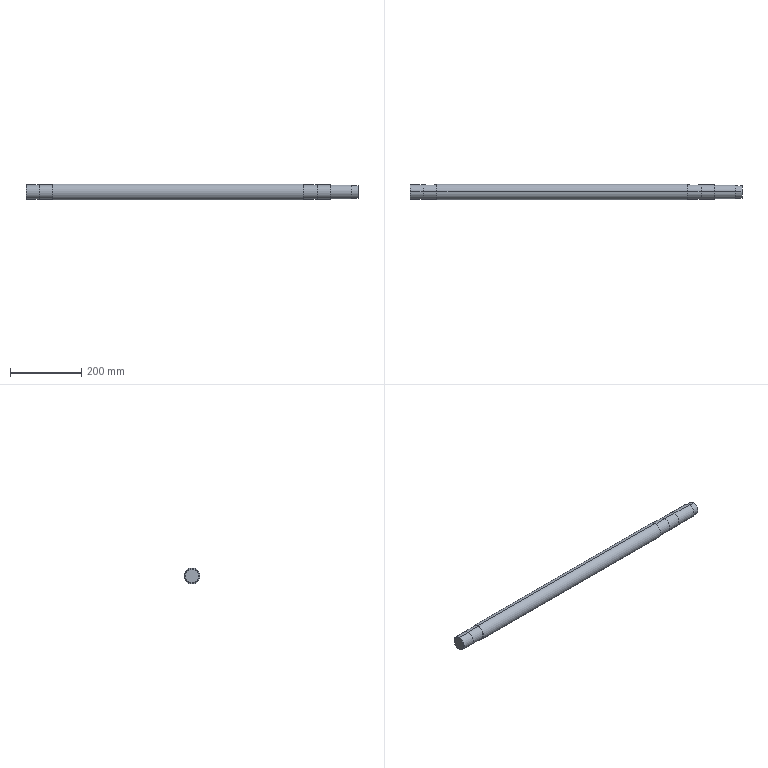Part | SolidWorks | features ICE 8, Chamfer 1, Extrusion 1, HoleWzd 1 | 1 solid | 43 faces | box 935 x 45 x 45 mm | volume 1400628 mm3 | cylinder 22 | plane 17 | cone 4 | commonest cylinder face diameters 12 x4 40 x4 41 x4 8.5 x2 10 x2 35 x2
STEP:
#1=CARTESIAN_POINT('',(844.,0.,4.25));
#2=VERTEX_POINT('',#1);
#3=CARTESIAN_POINT('',(844.,0.,-4.25));
#4=VERTEX_POINT('',#3);
#5=CARTESIAN_POINT('',(844.,0.,0.));
#6=DIRECTION('',(1.,0.,0.));
#7=DIRECTION('',(0.,0.,-1.));
#8=AXIS2_PLACEMENT_3D('',#5,#6,#7);
#9=CIRCLE('',#8,4.25);
#10=EDGE_CURVE('',#2,#4,#9,.T.);
#11=ORIENTED_EDGE('',*,*,#10,.F.);
#12=CARTESIAN_POINT('',(859.,0.,4.25));
#13=VERTEX_POINT('',#12);
#14=CARTESIAN_POINT('',(859.,0.,4.25));
#15=DIRECTION('',(1.,0.,0.));
#16=VECTOR('',#15,1000.);
#17=LINE('',#14,#16);
#18=EDGE_CURVE('',#2,#13,#17,.T.);
#19=ORIENTED_EDGE('',*,*,#18,.T.);
#20=CARTESIAN_POINT('',(859.,0.,-4.25));
#21=VERTEX_POINT('',#20);
#22=CARTESIAN_POINT('',(859.,0.,0.));
#23=DIRECTION('',(1.,0.,0.));
#24=DIRECTION('',(0.,0.,-1.));
#25=AXIS2_PLACEMENT_3D('',#22,#23,#24);
#26=CIRCLE('',#25,4.25);
#27=EDGE_CURVE('',#13,#21,#26,.T.);
#28=ORIENTED_EDGE('',*,*,#27,.T.);
#29=CARTESIAN_POINT('',(859.,0.,-4.25));
#30=DIRECTION('',(1.,0.,0.));
#31=VECTOR('',#30,1000.);
#32=LINE('',#29,#31);
#33=EDGE_CURVE('',#4,#21,#32,.T.);
#34=ORIENTED_EDGE('',*,*,#33,.F.);
#35=EDGE_LOOP('',(#11,#19,#28,#34));
#36=FACE_OUTER_BOUND('',#35,.T.);
#37=CARTESIAN_POINT('',(859.,0.,0.));
#38=DIRECTION('',(1.,0.,0.));
#39=DIRECTION('',(0.,0.,-1.));
#40=AXIS2_PLACEMENT_3D('',#37,#38,#39);
#41=CYLINDRICAL_SURFACE('',#40,4.25);
#42=ADVANCED_FACE('',(#36),#41,.F.);
#43=CARTESIAN_POINT('',(841.446,0.,0.));
#44=VERTEX_POINT('',#43);
#45=CARTESIAN_POINT('',(844.,0.,-4.25));
#46=DIRECTION('',(0.515,0.,-0.8572));
#47=VECTOR('',#46,1000.);
#48=LINE('',#45,#47);
#49=EDGE_CURVE('',#44,#4,#48,.T.);
#50=ORIENTED_EDGE('',*,*,#49,.F.);
#51=CARTESIAN_POINT('',(844.,0.,4.25));
#52=DIRECTION('',(0.515,0.,0.8572));
#53=VECTOR('',#52,1000.);
#54=LINE('',#51,#53);
#55=EDGE_CURVE('',#44,#2,#54,.T.);
#56=ORIENTED_EDGE('',*,*,#55,.T.);
#57=ORIENTED_EDGE('',*,*,#10,.T.);
#58=EDGE_LOOP('',(#50,#56,#57));
#59=FACE_OUTER_BOUND('',#58,.T.);
#60=CARTESIAN_POINT('',(844.,0.,0.));
#61=DIRECTION('',(1.,0.,0.));
#62=DIRECTION('',(0.,0.,-1.));
#63=AXIS2_PLACEMENT_3D('',#60,#61,#62);
#64=CONICAL_SURFACE('',#63,4.25,1.03);
#65=ADVANCED_FACE('',(#59),#64,.F.);
#66=CARTESIAN_POINT('',(-76.,0.,19.));
#67=VERTEX_POINT('',#66);
#68=CARTESIAN_POINT('',(-76.,0.,-19.));
#69=VERTEX_POINT('',#68);
#70=CARTESIAN_POINT('',(-76.,0.,0.));
#71=DIRECTION('',(-1.,0.,0.));
#72=DIRECTION('',(0.,0.,1.));
#73=AXIS2_PLACEMENT_3D('',#70,#71,#72);
#74=CIRCLE('',#73,19.);
#75=EDGE_CURVE('',#67,#69,#74,.T.);
#76=ORIENTED_EDGE('',*,*,#75,.F.);
#77=CARTESIAN_POINT('',(-75.,0.,20.));
#78=VERTEX_POINT('',#77);
#79=CARTESIAN_POINT('',(-76.,0.,19.));
#80=DIRECTION('',(0.7071,0.,0.7071));
#81=VECTOR('',#80,1000.);
#82=LINE('',#79,#81);
#83=EDGE_CURVE('',#67,#78,#82,.T.);
#84=ORIENTED_EDGE('',*,*,#83,.T.);
#85=CARTESIAN_POINT('',(-75.,0.,-20.));
#86=VERTEX_POINT('',#85);
#87=CARTESIAN_POINT('',(-75.,0.,0.));
#88=DIRECTION('',(1.,0.,0.));
#89=DIRECTION('',(0.,0.,1.));
#90=AXIS2_PLACEMENT_3D('',#87,#88,#89);
#91=CIRCLE('',#90,20.);
#92=EDGE_CURVE('',#86,#78,#91,.T.);
#93=ORIENTED_EDGE('',*,*,#92,.F.);
#94=CARTESIAN_POINT('',(-76.,0.,-19.));
#95=DIRECTION('',(0.7071,0.,-0.7071));
#96=VECTOR('',#95,1000.);
#97=LINE('',#94,#96);
#98=EDGE_CURVE('',#69,#86,#97,.T.);
#99=ORIENTED_EDGE('',*,*,#98,.F.);
#100=EDGE_LOOP('',(#76,#84,#93,#99));
#101=FACE_OUTER_BOUND('',#100,.T.);
#102=CARTESIAN_POINT('',(-76.,0.,0.));
#103=DIRECTION('',(1.,0.,0.));
#104=DIRECTION('',(0.,0.,-1.));
#105=AXIS2_PLACEMENT_3D('',#102,#103,#104);
#106=CONICAL_SURFACE('',#105,19.,0.7854);
#107=ADVANCED_FACE('',(#101),#106,.T.);
#108=ORIENTED_EDGE('',*,*,#92,.T.);
#109=CARTESIAN_POINT('',(-39.,0.,20.));
#110=VERTEX_POINT('',#109);
#111=CARTESIAN_POINT('',(-76.,0.,20.));
#112=DIRECTION('',(1.,0.,0.));
#113=VECTOR('',#112,1000.);
#114=LINE('',#111,#113);
#115=EDGE_CURVE('',#78,#110,#114,.T.);
#116=ORIENTED_EDGE('',*,*,#115,.T.);
#117=CARTESIAN_POINT('',(-39.,0.,-20.));
#118=VERTEX_POINT('',#117);
#119=CARTESIAN_POINT('',(-39.,0.,0.));
#120=DIRECTION('',(-1.,0.,0.));
#121=DIRECTION('',(0.,0.,1.));
#122=AXIS2_PLACEMENT_3D('',#119,#120,#121);
#123=CIRCLE('',#122,20.);
#124=EDGE_CURVE('',#110,#118,#123,.T.);
#125=ORIENTED_EDGE('',*,*,#124,.T.);
#126=CARTESIAN_POINT('',(-76.,0.,-20.));
#127=DIRECTION('',(1.,0.,0.));
#128=VECTOR('',#127,1000.);
#129=LINE('',#126,#128);
#130=EDGE_CURVE('',#86,#118,#129,.T.);
#131=ORIENTED_EDGE('',*,*,#130,.F.);
#132=EDGE_LOOP('',(#108,#116,#125,#131));
#133=FACE_OUTER_BOUND('',#132,.T.);
#134=CARTESIAN_POINT('',(-76.,0.,0.));
#135=DIRECTION('',(1.,0.,0.));
#136=DIRECTION('',(0.,0.,-1.));
#137=AXIS2_PLACEMENT_3D('',#134,#135,#136);
#138=CYLINDRICAL_SURFACE('',#137,20.);
#139=ADVANCED_FACE('',(#133),#138,.T.);
#140=CARTESIAN_POINT('',(-10.,19.602,6.));
#141=VERTEX_POINT('',#140);
#142=CARTESIAN_POINT('',(-30.,19.602,6.));
#143=VERTEX_POINT('',#142);
#144=CARTESIAN_POINT('',(-39.,19.602,6.));
#145=DIRECTION('',(-1.,0.,0.));
#146=VECTOR('',#145,1000.);
#147=LINE('',#144,#146);
#148=EDGE_CURVE('',#141,#143,#147,.T.);
#149=ORIENTED_EDGE('',*,*,#148,.T.);
#150=CARTESIAN_POINT('',(-30.,19.602,-6.));
#151=VERTEX_POINT('',#150);
#152=CARTESIAN_POINT('',(-30.,19.602,6.));
#153=CARTESIAN_POINT('',(-30.399,19.602,6.));
#154=CARTESIAN_POINT('',(-30.79,19.614,5.961));
#155=CARTESIAN_POINT('',(-31.367,19.649,5.845));
#156=CARTESIAN_POINT('',(-31.558,19.663,5.798));
#157=CARTESIAN_POINT('',(-31.936,19.697,5.683));
#158=CARTESIAN_POINT('',(-32.123,19.716,5.615));
#159=CARTESIAN_POINT('',(-32.667,19.78,5.389));
#160=CARTESIAN_POINT('',(-33.011,19.83,5.205));
#161=CARTESIAN_POINT('',(-33.499,19.911,4.878));
#162=CARTESIAN_POINT('',(-33.657,19.94,4.76));
#163=CARTESIAN_POINT('',(-33.96,19.998,4.511));
#164=CARTESIAN_POINT('',(-34.105,20.027,4.38));
#165=CARTESIAN_POINT('',(-34.517,20.114,3.968));
#166=CARTESIAN_POINT('',(-34.765,20.172,3.667));
#167=CARTESIAN_POINT('',(-35.204,20.28,3.012));
#168=CARTESIAN_POINT('',(-35.389,20.329,2.667));
#169=CARTESIAN_POINT('',(-35.614,20.39,2.126));
#170=CARTESIAN_POINT('',(-35.68,20.409,1.942));
#171=CARTESIAN_POINT('',(-35.796,20.441,1.565));
#172=CARTESIAN_POINT('',(-35.844,20.455,1.372));
#173=CARTESIAN_POINT('',(-35.961,20.488,0.7902));
#174=CARTESIAN_POINT('',(-36.,20.5,0.3995));
#175=CARTESIAN_POINT('',(-36.,20.5,-0.3879));
#176=CARTESIAN_POINT('',(-35.961,20.488,-0.7878));
#177=CARTESIAN_POINT('',(-35.807,20.444,-1.559));
#178=CARTESIAN_POINT('',(-35.693,20.412,-1.934));
#179=CARTESIAN_POINT('',(-35.466,20.35,-2.481));
#180=CARTESIAN_POINT('',(-35.382,20.327,-2.66));
#181=CARTESIAN_POINT('',(-35.196,20.279,-3.006));
#182=CARTESIAN_POINT('',(-35.096,20.254,-3.173));
#183=CARTESIAN_POINT('',(-34.879,20.2,-3.497));
#184=CARTESIAN_POINT('',(-34.763,20.172,-3.654));
#185=CARTESIAN_POINT('',(-34.515,20.115,-3.956));
#186=CARTESIAN_POINT('',(-34.383,20.086,-4.103));
#187=CARTESIAN_POINT('',(-33.967,19.998,-4.518));
#188=CARTESIAN_POINT('',(-33.667,19.94,-4.765));
#189=CARTESIAN_POINT('',(-33.019,19.831,-5.2));
#190=CARTESIAN_POINT('',(-32.668,19.78,-5.388));
#191=CARTESIAN_POINT('',(-31.945,19.695,-5.689));
#192=CARTESIAN_POINT('',(-31.571,19.661,-5.804));
#193=CARTESIAN_POINT('',(-30.797,19.615,-5.96));
#194=CARTESIAN_POINT('',(-30.399,19.602,-6.));
#195=CARTESIAN_POINT('',(-30.,19.602,-6.));
#196=B_SPLINE_CURVE_WITH_KNOTS('',3,(#152,#153,#154,#155,#156,#157,#158,#159,#160,#161,#162,#163,#164,#165,#166,#167,#168,#169,#170,#171,#172,#173,#174,#175,#176,#177,#178,#179,#180,#181,#182,#183,#184,#185,#186,#187,#188,#189,#190,#191,#192,#193,#194,#195),.UNSPECIFIED.,.F.,.F.,(4,2,2,2,2,2,2,2,2,2,2,2,2,2,2,2,2,2,2,2,2,4),(0.,0.001178,0.001768,0.002357,0.003535,0.004125,0.004714,0.005892,0.007071,0.00766,0.008249,0.009428,0.01061,0.01178,0.01237,0.01296,0.01355,0.01414,0.01532,0.0165,0.01768,0.01886),.UNSPECIFIED.);
#197=EDGE_CURVE('',#143,#151,#196,.T.);
#198=ORIENTED_EDGE('',*,*,#197,.T.);
#199=CARTESIAN_POINT('',(-10.,19.602,-6.));
#200=VERTEX_POINT('',#199);
#201=CARTESIAN_POINT('',(-39.,19.602,-6.));
#202=DIRECTION('',(1.,0.,0.));
#203=VECTOR('',#202,1000.);
#204=LINE('',#201,#203);
#205=EDGE_CURVE('',#151,#200,#204,.T.);
#206=ORIENTED_EDGE('',*,*,#205,.T.);
#207=CARTESIAN_POINT('',(-10.,19.602,-6.));
#208=CARTESIAN_POINT('',(-9.607,19.602,-6.));
#209=CARTESIAN_POINT('',(-9.214,19.614,-5.961));
#210=CARTESIAN_POINT('',(-8.435,19.661,-5.806));
#211=CARTESIAN_POINT('',(-8.059,19.695,-5.691));
#212=CARTESIAN_POINT('',(-7.336,19.779,-5.391));
#213=CARTESIAN_POINT('',(-6.985,19.83,-5.202));
#214=CARTESIAN_POINT('',(-6.336,19.939,-4.768));
#215=CARTESIAN_POINT('',(-6.036,19.997,-4.521));
#216=CARTESIAN_POINT('',(-5.62,20.085,-4.106));
#217=CARTESIAN_POINT('',(-5.487,20.115,-3.959));
#218=CARTESIAN_POINT('',(-5.239,20.172,-3.656));
#219=CARTESIAN_POINT('',(-5.123,20.2,-3.5));
#220=CARTESIAN_POINT('',(-4.798,20.28,-3.015));
#221=CARTESIAN_POINT('',(-4.612,20.329,-2.671));
#222=CARTESIAN_POINT('',(-4.308,20.411,-1.939));
#223=CARTESIAN_POINT('',(-4.194,20.444,-1.563));
#224=CARTESIAN_POINT('',(-4.078,20.477,-0.9866));
#225=CARTESIAN_POINT('',(-4.049,20.486,-0.7921));
#226=CARTESIAN_POINT('',(-4.01,20.497,-0.3983));
#227=CARTESIAN_POINT('',(-4.,20.5,-0.1983));
#228=CARTESIAN_POINT('',(-4.,20.5,0.3949));
#229=CARTESIAN_POINT('',(-4.039,20.489,0.7858));
#230=CARTESIAN_POINT('',(-4.193,20.444,1.559));
#231=CARTESIAN_POINT('',(-4.309,20.411,1.941));
#232=CARTESIAN_POINT('',(-4.61,20.329,2.664));
#233=CARTESIAN_POINT('',(-4.794,20.281,3.009));
#234=CARTESIAN_POINT('',(-5.233,20.172,3.665));
#235=CARTESIAN_POINT('',(-5.481,20.115,3.966));
#236=CARTESIAN_POINT('',(-5.894,20.027,4.379));
#237=CARTESIAN_POINT('',(-6.038,19.998,4.51));
#238=CARTESIAN_POINT('',(-6.341,19.94,4.759));
#239=CARTESIAN_POINT('',(-6.5,19.912,4.877));
#240=CARTESIAN_POINT('',(-6.988,19.83,5.204));
#241=CARTESIAN_POINT('',(-7.331,19.78,5.388));
#242=CARTESIAN_POINT('',(-8.054,19.695,5.689));
#243=CARTESIAN_POINT('',(-8.437,19.661,5.806));
#244=CARTESIAN_POINT('',(-9.209,19.614,5.961));
#245=CARTESIAN_POINT('',(-9.601,19.602,6.));
#246=CARTESIAN_POINT('',(-10.,19.602,6.));
#247=B_SPLINE_CURVE_WITH_KNOTS('',3,(#207,#208,#209,#210,#211,#212,#213,#214,#215,#216,#217,#218,#219,#220,#221,#222,#223,#224,#225,#226,#227,#228,#229,#230,#231,#232,#233,#234,#235,#236,#237,#238,#239,#240,#241,#242,#243,#244,#245,#246),.UNSPECIFIED.,.F.,.F.,(4,2,2,2,2,2,2,2,2,2,2,2,2,2,2,2,2,2,2,4),(0.01886,0.02004,0.02122,0.0224,0.02358,0.02417,0.02476,0.02593,0.02711,0.0277,0.02829,0.02947,0.03065,0.03183,0.03301,0.03359,0.03418,0.03536,0.03654,0.03772),.UNSPECIFIED.);
#248=EDGE_CURVE('',#200,#141,#247,.T.);
#249=ORIENTED_EDGE('',*,*,#248,.T.);
#250=EDGE_LOOP('',(#149,#198,#206,#249));
#251=FACE_BOUND('',#250,.T.);
#252=CARTESIAN_POINT('',(-39.,0.,20.5));
#253=VERTEX_POINT('',#252);
#254=CARTESIAN_POINT('',(-39.,0.,-20.5));
#255=VERTEX_POINT('',#254);
#256=CARTESIAN_POINT('',(-39.,0.,0.));
#257=DIRECTION('',(-1.,0.,0.));
#258=DIRECTION('',(0.,0.,1.));
#259=AXIS2_PLACEMENT_3D('',#256,#257,#258);
#260=CIRCLE('',#259,20.5);
#261=EDGE_CURVE('',#253,#255,#260,.T.);
#262=ORIENTED_EDGE('',*,*,#261,.F.);
#263=CARTESIAN_POINT('',(0.,0.,20.5));
#264=VERTEX_POINT('',#263);
#265=CARTESIAN_POINT('',(-39.,0.,20.5));
#266=DIRECTION('',(1.,0.,0.));
#267=VECTOR('',#266,1000.);
#268=LINE('',#265,#267);
#269=EDGE_CURVE('',#253,#264,#268,.T.);
#270=ORIENTED_EDGE('',*,*,#269,.T.);
#271=CARTESIAN_POINT('',(0.,0.,-20.5));
#272=VERTEX_POINT('',#271);
#273=CARTESIAN_POINT('',(0.,0.,0.));
#274=DIRECTION('',(-1.,0.,0.));
#275=DIRECTION('',(0.,0.,-1.));
#276=AXIS2_PLACEMENT_3D('',#273,#274,#275);
#277=CIRCLE('',#276,20.5);
#278=EDGE_CURVE('',#264,#272,#277,.T.);
#279=ORIENTED_EDGE('',*,*,#278,.T.);
#280=CARTESIAN_POINT('',(-39.,0.,-20.5));
#281=DIRECTION('',(1.,0.,0.));
#282=VECTOR('',#281,1000.);
#283=LINE('',#280,#282);
#284=EDGE_CURVE('',#255,#272,#283,.T.);
#285=ORIENTED_EDGE('',*,*,#284,.F.);
#286=EDGE_LOOP('',(#262,#270,#279,#285));
#287=FACE_OUTER_BOUND('',#286,.T.);
#288=CARTESIAN_POINT('',(-39.,0.,0.));
#289=DIRECTION('',(1.,0.,0.));
#290=DIRECTION('',(0.,0.,-1.));
#291=AXIS2_PLACEMENT_3D('',#288,#289,#290);
#292=CYLINDRICAL_SURFACE('',#291,20.5);
#293=ADVANCED_FACE('',(#251,#287),#292,.T.);
#294=CARTESIAN_POINT('',(848.,16.771,-5.));
#295=VERTEX_POINT('',#294);
#296=CARTESIAN_POINT('',(852.,16.771,-5.));
#297=VERTEX_POINT('',#296);
#298=CARTESIAN_POINT('',(859.,16.771,-5.));
#299=DIRECTION('',(1.,0.,0.));
#300=VECTOR('',#299,1000.);
#301=LINE('',#298,#300);
#302=EDGE_CURVE('',#295,#297,#301,.T.);
#303=ORIENTED_EDGE('',*,*,#302,.T.);
#304=CARTESIAN_POINT('',(852.,16.771,5.));
#305=VERTEX_POINT('',#304);
#306=CARTESIAN_POINT('',(852.,16.771,-5.));
#307=CARTESIAN_POINT('',(852.332,16.771,-5.));
#308=CARTESIAN_POINT('',(852.658,16.78,-4.967));
#309=CARTESIAN_POINT('',(853.3,16.818,-4.839));
#310=CARTESIAN_POINT('',(853.618,16.846,-4.742));
#311=CARTESIAN_POINT('',(854.222,16.914,-4.491));
#312=CARTESIAN_POINT('',(854.509,16.955,-4.337));
#313=CARTESIAN_POINT('',(855.051,17.044,-3.975));
#314=CARTESIAN_POINT('',(855.306,17.092,-3.765));
#315=CARTESIAN_POINT('',(855.765,17.186,-3.306));
#316=CARTESIAN_POINT('',(855.971,17.233,-3.056));
#317=CARTESIAN_POINT('',(856.337,17.321,-2.51));
#318=CARTESIAN_POINT('',(856.491,17.361,-2.222));
#319=CARTESIAN_POINT('',(856.679,17.411,-1.771));
#320=CARTESIAN_POINT('',(856.734,17.426,-1.618));
#321=CARTESIAN_POINT('',(856.83,17.452,-1.304));
#322=CARTESIAN_POINT('',(856.87,17.463,-1.143));
#323=CARTESIAN_POINT('',(856.967,17.491,-0.6583));
#324=CARTESIAN_POINT('',(857.,17.5,-0.3328));
#325=CARTESIAN_POINT('',(857.,17.5,0.3232));
#326=CARTESIAN_POINT('',(856.968,17.491,0.6564));
#327=CARTESIAN_POINT('',(856.839,17.455,1.299));
#328=CARTESIAN_POINT('',(856.745,17.428,1.612));
#329=CARTESIAN_POINT('',(856.493,17.361,2.219));
#330=CARTESIAN_POINT('',(856.337,17.321,2.509));
#331=CARTESIAN_POINT('',(855.976,17.235,3.049));
#332=CARTESIAN_POINT('',(855.768,17.187,3.303));
#333=CARTESIAN_POINT('',(855.306,17.092,3.765));
#334=CARTESIAN_POINT('',(855.055,17.045,3.971));
#335=CARTESIAN_POINT('',(854.516,16.956,4.333));
#336=CARTESIAN_POINT('',(854.223,16.915,4.49));
#337=CARTESIAN_POINT('',(853.621,16.846,4.741));
#338=CARTESIAN_POINT('',(853.309,16.818,4.837));
#339=CARTESIAN_POINT('',(852.664,16.781,4.967));
#340=CARTESIAN_POINT('',(852.332,16.771,5.));
#341=CARTESIAN_POINT('',(852.,16.771,5.));
#342=B_SPLINE_CURVE_WITH_KNOTS('',3,(#306,#307,#308,#309,#310,#311,#312,#313,#314,#315,#316,#317,#318,#319,#320,#321,#322,#323,#324,#325,#326,#327,#328,#329,#330,#331,#332,#333,#334,#335,#336,#337,#338,#339,#340,#341),.UNSPECIFIED.,.F.,.F.,(4,2,2,2,2,2,2,2,2,2,2,2,2,2,2,2,2,4),(0.,0.0009818,0.001964,0.002945,0.003927,0.004909,0.005891,0.006382,0.006873,0.007855,0.008836,0.009818,0.0108,0.01178,0.01276,0.01375,0.01473,0.01571),.UNSPECIFIED.);
#343=EDGE_CURVE('',#297,#305,#342,.T.);
#344=ORIENTED_EDGE('',*,*,#343,.T.);
#345=CARTESIAN_POINT('',(848.,16.771,5.));
#346=VERTEX_POINT('',#345);
#347=CARTESIAN_POINT('',(859.,16.771,5.));
#348=DIRECTION('',(-1.,0.,0.));
#349=VECTOR('',#348,1000.);
#350=LINE('',#347,#349);
#351=EDGE_CURVE('',#305,#346,#350,.T.);
#352=ORIENTED_EDGE('',*,*,#351,.T.);
#353=CARTESIAN_POINT('',(848.,16.771,5.));
#354=CARTESIAN_POINT('',(847.668,16.771,5.));
#355=CARTESIAN_POINT('',(847.342,16.78,4.967));
#356=CARTESIAN_POINT('',(846.7,16.818,4.839));
#357=CARTESIAN_POINT('',(846.382,16.846,4.742));
#358=CARTESIAN_POINT('',(845.778,16.914,4.491));
#359=CARTESIAN_POINT('',(845.491,16.955,4.337));
#360=CARTESIAN_POINT('',(844.949,17.044,3.975));
#361=CARTESIAN_POINT('',(844.694,17.092,3.765));
#362=CARTESIAN_POINT('',(844.235,17.186,3.306));
#363=CARTESIAN_POINT('',(844.029,17.233,3.056));
#364=CARTESIAN_POINT('',(843.663,17.321,2.51));
#365=CARTESIAN_POINT('',(843.509,17.361,2.222));
#366=CARTESIAN_POINT('',(843.321,17.411,1.771));
#367=CARTESIAN_POINT('',(843.266,17.426,1.618));
#368=CARTESIAN_POINT('',(843.17,17.452,1.304));
#369=CARTESIAN_POINT('',(843.13,17.463,1.143));
#370=CARTESIAN_POINT('',(843.033,17.491,0.6583));
#371=CARTESIAN_POINT('',(843.,17.5,0.3328));
#372=CARTESIAN_POINT('',(843.,17.5,-0.3232));
#373=CARTESIAN_POINT('',(843.032,17.491,-0.6564));
#374=CARTESIAN_POINT('',(843.161,17.455,-1.299));
#375=CARTESIAN_POINT('',(843.255,17.428,-1.612));
#376=CARTESIAN_POINT('',(843.507,17.361,-2.219));
#377=CARTESIAN_POINT('',(843.663,17.321,-2.509));
#378=CARTESIAN_POINT('',(844.024,17.235,-3.049));
#379=CARTESIAN_POINT('',(844.232,17.187,-3.303));
#380=CARTESIAN_POINT('',(844.694,17.092,-3.765));
#381=CARTESIAN_POINT('',(844.945,17.045,-3.971));
#382=CARTESIAN_POINT('',(845.484,16.956,-4.333));
#383=CARTESIAN_POINT('',(845.777,16.915,-4.49));
#384=CARTESIAN_POINT('',(846.379,16.846,-4.741));
#385=CARTESIAN_POINT('',(846.691,16.818,-4.837));
#386=CARTESIAN_POINT('',(847.336,16.781,-4.967));
#387=CARTESIAN_POINT('',(847.668,16.771,-5.));
#388=CARTESIAN_POINT('',(848.,16.771,-5.));
#389=B_SPLINE_CURVE_WITH_KNOTS('',3,(#353,#354,#355,#356,#357,#358,#359,#360,#361,#362,#363,#364,#365,#366,#367,#368,#369,#370,#371,#372,#373,#374,#375,#376,#377,#378,#379,#380,#381,#382,#383,#384,#385,#386,#387,#388),.UNSPECIFIED.,.F.,.F.,(4,2,2,2,2,2,2,2,2,2,2,2,2,2,2,2,2,4),(0.,0.0009818,0.001964,0.002945,0.003927,0.004909,0.005891,0.006382,0.006873,0.007855,0.008836,0.009818,0.0108,0.01178,0.01276,0.01375,0.01473,0.01571),.UNSPECIFIED.);
#390=EDGE_CURVE('',#346,#295,#389,.T.);
#391=ORIENTED_EDGE('',*,*,#390,.T.);
#392=EDGE_LOOP('',(#303,#344,#352,#391));
#393=FACE_BOUND('',#392,.T.);
#394=CARTESIAN_POINT('',(859.,0.,-17.5));
#395=VERTEX_POINT('',#394);
#396=CARTESIAN_POINT('',(859.,0.,17.5));
#397=VERTEX_POINT('',#396);
#398=CARTESIAN_POINT('',(859.,0.,0.));
#399=DIRECTION('',(1.,0.,0.));
#400=DIRECTION('',(0.,0.,-1.));
#401=AXIS2_PLACEMENT_3D('',#398,#399,#400);
#402=CIRCLE('',#401,17.5);
#403=EDGE_CURVE('',#395,#397,#402,.T.);
#404=ORIENTED_EDGE('',*,*,#403,.F.);
#405=CARTESIAN_POINT('',(841.,0.,-17.5));
#406=VERTEX_POINT('',#405);
#407=CARTESIAN_POINT('',(859.,0.,-17.5));
#408=DIRECTION('',(-1.,0.,0.));
#409=VECTOR('',#408,1000.);
#410=LINE('',#407,#409);
#411=EDGE_CURVE('',#395,#406,#410,.T.);
#412=ORIENTED_EDGE('',*,*,#411,.T.);
#413=CARTESIAN_POINT('',(841.,0.,17.5));
#414=VERTEX_POINT('',#413);
#415=CARTESIAN_POINT('',(841.,0.,0.));
#416=DIRECTION('',(1.,0.,0.));
#417=DIRECTION('',(0.,0.,-1.));
#418=AXIS2_PLACEMENT_3D('',#415,#416,#417);
#419=CIRCLE('',#418,17.5);
#420=EDGE_CURVE('',#406,#414,#419,.T.);
#421=ORIENTED_EDGE('',*,*,#420,.T.);
#422=CARTESIAN_POINT('',(859.,0.,17.5));
#423=DIRECTION('',(-1.,0.,0.));
#424=VECTOR('',#423,1000.);
#425=LINE('',#422,#424);
#426=EDGE_CURVE('',#397,#414,#425,.T.);
#427=ORIENTED_EDGE('',*,*,#426,.F.);
#428=EDGE_LOOP('',(#404,#412,#421,#427));
#429=FACE_OUTER_BOUND('',#428,.T.);
#430=CARTESIAN_POINT('',(859.,0.,0.));
#431=DIRECTION('',(-1.,0.,0.));
#432=DIRECTION('',(0.,0.,1.));
#433=AXIS2_PLACEMENT_3D('',#430,#431,#432);
#434=CYLINDRICAL_SURFACE('',#433,17.5);
#435=ADVANCED_FACE('',(#393,#429),#434,.T.);
#436=CARTESIAN_POINT('',(841.,0.,-19.5));
#437=VERTEX_POINT('',#436);
#438=CARTESIAN_POINT('',(841.,0.,19.5));
#439=VERTEX_POINT('',#438);
#440=CARTESIAN_POINT('',(841.,0.,0.));
#441=DIRECTION('',(1.,0.,0.));
#442=DIRECTION('',(0.,0.,-1.));
#443=AXIS2_PLACEMENT_3D('',#440,#441,#442);
#444=CIRCLE('',#443,19.5);
#445=EDGE_CURVE('',#437,#439,#444,.T.);
#446=ORIENTED_EDGE('',*,*,#445,.F.);
#447=CARTESIAN_POINT('',(781.,0.,-19.5));
#448=VERTEX_POINT('',#447);
#449=CARTESIAN_POINT('',(841.,0.,-19.5));
#450=DIRECTION('',(-1.,0.,0.));
#451=VECTOR('',#450,1000.);
#452=LINE('',#449,#451);
#453=EDGE_CURVE('',#437,#448,#452,.T.);
#454=ORIENTED_EDGE('',*,*,#453,.T.);
#455=CARTESIAN_POINT('',(781.,0.,19.5));
#456=VERTEX_POINT('',#455);
#457=CARTESIAN_POINT('',(781.,0.,0.));
#458=DIRECTION('',(1.,0.,0.));
#459=DIRECTION('',(0.,0.,-1.));
#460=AXIS2_PLACEMENT_3D('',#457,#458,#459);
#461=CIRCLE('',#460,19.5);
#462=EDGE_CURVE('',#448,#456,#461,.T.);
#463=ORIENTED_EDGE('',*,*,#462,.T.);
#464=CARTESIAN_POINT('',(841.,0.,19.5));
#465=DIRECTION('',(-1.,0.,0.));
#466=VECTOR('',#465,1000.);
#467=LINE('',#464,#466);
#468=EDGE_CURVE('',#439,#456,#467,.T.);
#469=ORIENTED_EDGE('',*,*,#468,.F.);
#470=EDGE_LOOP('',(#446,#454,#463,#469));
#471=FACE_OUTER_BOUND('',#470,.T.);
#472=CARTESIAN_POINT('',(841.,0.,0.));
#473=DIRECTION('',(-1.,0.,0.));
#474=DIRECTION('',(0.,0.,1.));
#475=AXIS2_PLACEMENT_3D('',#472,#473,#474);
#476=CYLINDRICAL_SURFACE('',#475,19.5);
#477=ADVANCED_FACE('',(#471),#476,.T.);
#478=CARTESIAN_POINT('',(781.,0.,-20.));
#479=VERTEX_POINT('',#478);
#480=CARTESIAN_POINT('',(781.,0.,20.));
#481=VERTEX_POINT('',#480);
#482=CARTESIAN_POINT('',(781.,0.,0.));
#483=DIRECTION('',(1.,0.,0.));
#484=DIRECTION('',(0.,0.,-1.));
#485=AXIS2_PLACEMENT_3D('',#482,#483,#484);
#486=CIRCLE('',#485,20.);
#487=EDGE_CURVE('',#479,#481,#486,.T.);
#488=ORIENTED_EDGE('',*,*,#487,.F.);
#489=CARTESIAN_POINT('',(744.,0.,-20.));
#490=VERTEX_POINT('',#489);
#491=CARTESIAN_POINT('',(781.,0.,-20.));
#492=DIRECTION('',(-1.,0.,0.));
#493=VECTOR('',#492,1000.);
#494=LINE('',#491,#493);
#495=EDGE_CURVE('',#479,#490,#494,.T.);
#496=ORIENTED_EDGE('',*,*,#495,.T.);
#497=CARTESIAN_POINT('',(744.,0.,20.));
#498=VERTEX_POINT('',#497);
#499=CARTESIAN_POINT('',(744.,0.,0.));
#500=DIRECTION('',(1.,0.,0.));
#501=DIRECTION('',(0.,0.,-1.));
#502=AXIS2_PLACEMENT_3D('',#499,#500,#501);
#503=CIRCLE('',#502,20.);
#504=EDGE_CURVE('',#490,#498,#503,.T.);
#505=ORIENTED_EDGE('',*,*,#504,.T.);
#506=CARTESIAN_POINT('',(781.,0.,20.));
#507=DIRECTION('',(-1.,0.,0.));
#508=VECTOR('',#507,1000.);
#509=LINE('',#506,#508);
#510=EDGE_CURVE('',#481,#498,#509,.T.);
#511=ORIENTED_EDGE('',*,*,#510,.F.);
#512=EDGE_LOOP('',(#488,#496,#505,#511));
#513=FACE_OUTER_BOUND('',#512,.T.);
#514=CARTESIAN_POINT('',(781.,0.,0.));
#515=DIRECTION('',(-1.,0.,0.));
#516=DIRECTION('',(0.,0.,1.));
#517=AXIS2_PLACEMENT_3D('',#514,#515,#516);
#518=CYLINDRICAL_SURFACE('',#517,20.);
#519=ADVANCED_FACE('',(#513),#518,.T.);
#520=CARTESIAN_POINT('',(715.,19.602,-6.));
#521=VERTEX_POINT('',#520);
#522=CARTESIAN_POINT('',(735.,19.602,-6.));
#523=VERTEX_POINT('',#522);
#524=CARTESIAN_POINT('',(744.,19.602,-6.));
#525=DIRECTION('',(1.,0.,0.));
#526=VECTOR('',#525,1000.);
#527=LINE('',#524,#526);
#528=EDGE_CURVE('',#521,#523,#527,.T.);
#529=ORIENTED_EDGE('',*,*,#528,.T.);
#530=CARTESIAN_POINT('',(735.,19.602,6.));
#531=VERTEX_POINT('',#530);
#532=CARTESIAN_POINT('',(735.,19.602,-6.));
#533=CARTESIAN_POINT('',(735.393,19.602,-6.));
#534=CARTESIAN_POINT('',(735.786,19.614,-5.961));
#535=CARTESIAN_POINT('',(736.565,19.661,-5.806));
#536=CARTESIAN_POINT('',(736.941,19.695,-5.691));
#537=CARTESIAN_POINT('',(737.664,19.779,-5.391));
#538=CARTESIAN_POINT('',(738.015,19.83,-5.202));
#539=CARTESIAN_POINT('',(738.664,19.939,-4.768));
#540=CARTESIAN_POINT('',(738.964,19.997,-4.521));
#541=CARTESIAN_POINT('',(739.38,20.085,-4.106));
#542=CARTESIAN_POINT('',(739.513,20.115,-3.959));
#543=CARTESIAN_POINT('',(739.761,20.172,-3.656));
#544=CARTESIAN_POINT('',(739.877,20.2,-3.5));
#545=CARTESIAN_POINT('',(740.202,20.28,-3.015));
#546=CARTESIAN_POINT('',(740.388,20.329,-2.671));
#547=CARTESIAN_POINT('',(740.692,20.411,-1.939));
#548=CARTESIAN_POINT('',(740.806,20.444,-1.563));
#549=CARTESIAN_POINT('',(740.922,20.477,-0.9866));
#550=CARTESIAN_POINT('',(740.951,20.486,-0.7921));
#551=CARTESIAN_POINT('',(740.99,20.497,-0.3983));
#552=CARTESIAN_POINT('',(741.,20.5,-0.1983));
#553=CARTESIAN_POINT('',(741.,20.5,0.3949));
#554=CARTESIAN_POINT('',(740.961,20.489,0.7858));
#555=CARTESIAN_POINT('',(740.807,20.444,1.559));
#556=CARTESIAN_POINT('',(740.691,20.411,1.941));
#557=CARTESIAN_POINT('',(740.39,20.329,2.664));
#558=CARTESIAN_POINT('',(740.206,20.281,3.009));
#559=CARTESIAN_POINT('',(739.767,20.172,3.665));
#560=CARTESIAN_POINT('',(739.519,20.115,3.966));
#561=CARTESIAN_POINT('',(739.106,20.027,4.379));
#562=CARTESIAN_POINT('',(738.962,19.998,4.51));
#563=CARTESIAN_POINT('',(738.659,19.94,4.759));
#564=CARTESIAN_POINT('',(738.5,19.912,4.877));
#565=CARTESIAN_POINT('',(738.012,19.83,5.204));
#566=CARTESIAN_POINT('',(737.669,19.78,5.388));
#567=CARTESIAN_POINT('',(736.946,19.695,5.689));
#568=CARTESIAN_POINT('',(736.563,19.661,5.806));
#569=CARTESIAN_POINT('',(735.791,19.614,5.961));
#570=CARTESIAN_POINT('',(735.399,19.602,6.));
#571=CARTESIAN_POINT('',(735.,19.602,6.));
#572=B_SPLINE_CURVE_WITH_KNOTS('',3,(#532,#533,#534,#535,#536,#537,#538,#539,#540,#541,#542,#543,#544,#545,#546,#547,#548,#549,#550,#551,#552,#553,#554,#555,#556,#557,#558,#559,#560,#561,#562,#563,#564,#565,#566,#567,#568,#569,#570,#571),.UNSPECIFIED.,.F.,.F.,(4,2,2,2,2,2,2,2,2,2,2,2,2,2,2,2,2,2,2,4),(0.01886,0.02004,0.02122,0.0224,0.02358,0.02417,0.02476,0.02593,0.02711,0.0277,0.02829,0.02947,0.03065,0.03183,0.03301,0.03359,0.03418,0.03536,0.03654,0.03772),.UNSPECIFIED.);
#573=EDGE_CURVE('',#523,#531,#572,.T.);
#574=ORIENTED_EDGE('',*,*,#573,.T.);
#575=CARTESIAN_POINT('',(715.,19.602,6.));
#576=VERTEX_POINT('',#575);
#577=CARTESIAN_POINT('',(744.,19.602,6.));
#578=DIRECTION('',(-1.,0.,0.));
#579=VECTOR('',#578,1000.);
#580=LINE('',#577,#579);
#581=EDGE_CURVE('',#531,#576,#580,.T.);
#582=ORIENTED_EDGE('',*,*,#581,.T.);
#583=CARTESIAN_POINT('',(715.,19.602,6.));
#584=CARTESIAN_POINT('',(714.601,19.602,6.));
#585=CARTESIAN_POINT('',(714.21,19.614,5.961));
#586=CARTESIAN_POINT('',(713.633,19.649,5.845));
#587=CARTESIAN_POINT('',(713.442,19.663,5.798));
#588=CARTESIAN_POINT('',(713.064,19.697,5.683));
#589=CARTESIAN_POINT('',(712.877,19.716,5.615));
#590=CARTESIAN_POINT('',(712.333,19.78,5.389));
#591=CARTESIAN_POINT('',(711.989,19.83,5.205));
#592=CARTESIAN_POINT('',(711.501,19.911,4.878));
#593=CARTESIAN_POINT('',(711.343,19.94,4.76));
#594=CARTESIAN_POINT('',(711.04,19.998,4.511));
#595=CARTESIAN_POINT('',(710.895,20.027,4.38));
#596=CARTESIAN_POINT('',(710.483,20.114,3.968));
#597=CARTESIAN_POINT('',(710.235,20.172,3.667));
#598=CARTESIAN_POINT('',(709.796,20.28,3.012));
#599=CARTESIAN_POINT('',(709.611,20.329,2.667));
#600=CARTESIAN_POINT('',(709.386,20.39,2.126));
#601=CARTESIAN_POINT('',(709.32,20.409,1.942));
#602=CARTESIAN_POINT('',(709.204,20.441,1.565));
#603=CARTESIAN_POINT('',(709.156,20.455,1.372));
#604=CARTESIAN_POINT('',(709.039,20.488,0.7902));
#605=CARTESIAN_POINT('',(709.,20.5,0.3995));
#606=CARTESIAN_POINT('',(709.,20.5,-0.3879));
#607=CARTESIAN_POINT('',(709.039,20.488,-0.7878));
#608=CARTESIAN_POINT('',(709.193,20.444,-1.559));
#609=CARTESIAN_POINT('',(709.307,20.412,-1.934));
#610=CARTESIAN_POINT('',(709.534,20.35,-2.481));
#611=CARTESIAN_POINT('',(709.618,20.327,-2.66));
#612=CARTESIAN_POINT('',(709.804,20.279,-3.006));
#613=CARTESIAN_POINT('',(709.904,20.254,-3.173));
#614=CARTESIAN_POINT('',(710.121,20.2,-3.497));
#615=CARTESIAN_POINT('',(710.237,20.172,-3.654));
#616=CARTESIAN_POINT('',(710.485,20.115,-3.956));
#617=CARTESIAN_POINT('',(710.617,20.086,-4.103));
#618=CARTESIAN_POINT('',(711.033,19.998,-4.518));
#619=CARTESIAN_POINT('',(711.333,19.94,-4.765));
#620=CARTESIAN_POINT('',(711.981,19.831,-5.2));
#621=CARTESIAN_POINT('',(712.332,19.78,-5.388));
#622=CARTESIAN_POINT('',(713.055,19.695,-5.689));
#623=CARTESIAN_POINT('',(713.429,19.661,-5.804));
#624=CARTESIAN_POINT('',(714.203,19.615,-5.96));
#625=CARTESIAN_POINT('',(714.601,19.602,-6.));
#626=CARTESIAN_POINT('',(715.,19.602,-6.));
#627=B_SPLINE_CURVE_WITH_KNOTS('',3,(#583,#584,#585,#586,#587,#588,#589,#590,#591,#592,#593,#594,#595,#596,#597,#598,#599,#600,#601,#602,#603,#604,#605,#606,#607,#608,#609,#610,#611,#612,#613,#614,#615,#616,#617,#618,#619,#620,#621,#622,#623,#624,#625,#626),.UNSPECIFIED.,.F.,.F.,(4,2,2,2,2,2,2,2,2,2,2,2,2,2,2,2,2,2,2,2,2,4),(0.,0.001178,0.001768,0.002357,0.003535,0.004125,0.004714,0.005892,0.007071,0.00766,0.008249,0.009428,0.01061,0.01178,0.01237,0.01296,0.01355,0.01414,0.01532,0.0165,0.01768,0.01886),.UNSPECIFIED.);
#628=EDGE_CURVE('',#576,#521,#627,.T.);
#629=ORIENTED_EDGE('',*,*,#628,.T.);
#630=EDGE_LOOP('',(#529,#574,#582,#629));
#631=FACE_BOUND('',#630,.T.);
#632=CARTESIAN_POINT('',(744.,0.,-20.5));
#633=VERTEX_POINT('',#632);
#634=CARTESIAN_POINT('',(744.,0.,20.5));
#635=VERTEX_POINT('',#634);
#636=CARTESIAN_POINT('',(744.,0.,0.));
#637=DIRECTION('',(1.,0.,0.));
#638=DIRECTION('',(0.,0.,-1.));
#639=AXIS2_PLACEMENT_3D('',#636,#637,#638);
#640=CIRCLE('',#639,20.5);
#641=EDGE_CURVE('',#633,#635,#640,.T.);
#642=ORIENTED_EDGE('',*,*,#641,.F.);
#643=CARTESIAN_POINT('',(705.,0.,-20.5));
#644=VERTEX_POINT('',#643);
#645=CARTESIAN_POINT('',(744.,0.,-20.5));
#646=DIRECTION('',(-1.,0.,0.));
#647=VECTOR('',#646,1000.);
#648=LINE('',#645,#647);
#649=EDGE_CURVE('',#633,#644,#648,.T.);
#650=ORIENTED_EDGE('',*,*,#649,.T.);
#651=CARTESIAN_POINT('',(705.,0.,20.5));
#652=VERTEX_POINT('',#651);
#653=CARTESIAN_POINT('',(705.,0.,0.));
#654=DIRECTION('',(1.,0.,0.));
#655=DIRECTION('',(0.,0.,-1.));
#656=AXIS2_PLACEMENT_3D('',#653,#654,#655);
#657=CIRCLE('',#656,20.5);
#658=EDGE_CURVE('',#644,#652,#657,.T.);
#659=ORIENTED_EDGE('',*,*,#658,.T.);
#660=CARTESIAN_POINT('',(744.,0.,20.5));
#661=DIRECTION('',(-1.,0.,0.));
#662=VECTOR('',#661,1000.);
#663=LINE('',#660,#662);
#664=EDGE_CURVE('',#635,#652,#663,.T.);
#665=ORIENTED_EDGE('',*,*,#664,.F.);
#666=EDGE_LOOP('',(#642,#650,#659,#665));
#667=FACE_OUTER_BOUND('',#666,.T.);
#668=CARTESIAN_POINT('',(744.,0.,0.));
#669=DIRECTION('',(-1.,0.,0.));
#670=DIRECTION('',(0.,0.,1.));
#671=AXIS2_PLACEMENT_3D('',#668,#669,#670);
#672=CYLINDRICAL_SURFACE('',#671,20.5);
#673=ADVANCED_FACE('',(#631,#667),#672,.T.);
#674=CARTESIAN_POINT('',(705.,0.,-22.5));
#675=VERTEX_POINT('',#674);
#676=CARTESIAN_POINT('',(705.,0.,22.5));
#677=VERTEX_POINT('',#676);
#678=CARTESIAN_POINT('',(705.,0.,0.));
#679=DIRECTION('',(1.,0.,0.));
#680=DIRECTION('',(0.,0.,-1.));
#681=AXIS2_PLACEMENT_3D('',#678,#679,#680);
#682=CIRCLE('',#681,22.5);
#683=EDGE_CURVE('',#675,#677,#682,.T.);
#684=ORIENTED_EDGE('',*,*,#683,.F.);
#685=CARTESIAN_POINT('',(0.,0.,-22.5));
#686=VERTEX_POINT('',#685);
#687=CARTESIAN_POINT('',(705.,0.,-22.5));
#688=DIRECTION('',(-1.,0.,0.));
#689=VECTOR('',#688,1000.);
#690=LINE('',#687,#689);
#691=EDGE_CURVE('',#675,#686,#690,.T.);
#692=ORIENTED_EDGE('',*,*,#691,.T.);
#693=CARTESIAN_POINT('',(0.,0.,22.5));
#694=VERTEX_POINT('',#693);
#695=CARTESIAN_POINT('',(0.,0.,0.));
#696=DIRECTION('',(1.,0.,0.));
#697=DIRECTION('',(0.,0.,-1.));
#698=AXIS2_PLACEMENT_3D('',#695,#696,#697);
#699=CIRCLE('',#698,22.5);
#700=EDGE_CURVE('',#686,#694,#699,.T.);
#701=ORIENTED_EDGE('',*,*,#700,.T.);
#702=CARTESIAN_POINT('',(705.,0.,22.5));
#703=DIRECTION('',(-1.,0.,0.));
#704=VECTOR('',#703,1000.);
#705=LINE('',#702,#704);
#706=EDGE_CURVE('',#677,#694,#705,.T.);
#707=ORIENTED_EDGE('',*,*,#706,.F.);
#708=EDGE_LOOP('',(#684,#692,#701,#707));
#709=FACE_OUTER_BOUND('',#708,.T.);
#710=CARTESIAN_POINT('',(705.,0.,0.));
#711=DIRECTION('',(-1.,0.,0.));
#712=DIRECTION('',(0.,0.,1.));
#713=AXIS2_PLACEMENT_3D('',#710,#711,#712);
#714=CYLINDRICAL_SURFACE('',#713,22.5);
#715=ADVANCED_FACE('',(#709),#714,.T.);
#716=CARTESIAN_POINT('',(-39.,0.,0.));
#717=DIRECTION('',(-1.,0.,0.));
#718=DIRECTION('',(0.,0.,1.));
#719=AXIS2_PLACEMENT_3D('',#716,#717,#718);
#720=CIRCLE('',#719,20.5);
#721=EDGE_CURVE('',#255,#253,#720,.T.);
#722=ORIENTED_EDGE('',*,*,#721,.T.);
#723=ORIENTED_EDGE('',*,*,#261,.T.);
#724=EDGE_LOOP('',(#722,#723));
#725=FACE_OUTER_BOUND('',#724,.T.);
#726=CARTESIAN_POINT('',(-39.,0.,0.));
#727=DIRECTION('',(-1.,0.,0.));
#728=DIRECTION('',(0.,0.,1.));
#729=AXIS2_PLACEMENT_3D('',#726,#727,#728);
#730=CIRCLE('',#729,20.);
#731=EDGE_CURVE('',#118,#110,#730,.T.);
#732=ORIENTED_EDGE('',*,*,#731,.F.);
#733=ORIENTED_EDGE('',*,*,#124,.F.);
#734=EDGE_LOOP('',(#732,#733));
#735=FACE_BOUND('',#734,.T.);
#736=CARTESIAN_POINT('',(-39.,0.,0.));
#737=DIRECTION('',(-1.,0.,0.));
#738=DIRECTION('',(0.,0.,1.));
#739=AXIS2_PLACEMENT_3D('',#736,#737,#738);
#740=PLANE('',#739);
#741=ADVANCED_FACE('',(#725,#735),#740,.T.);
#742=CARTESIAN_POINT('',(0.,0.,0.));
#743=DIRECTION('',(1.,0.,0.));
#744=DIRECTION('',(0.,0.,-1.));
#745=AXIS2_PLACEMENT_3D('',#742,#743,#744);
#746=CIRCLE('',#745,22.5);
#747=EDGE_CURVE('',#694,#686,#746,.T.);
#748=ORIENTED_EDGE('',*,*,#747,.F.);
#749=ORIENTED_EDGE('',*,*,#700,.F.);
#750=EDGE_LOOP('',(#748,#749));
#751=FACE_OUTER_BOUND('',#750,.T.);
#752=CARTESIAN_POINT('',(0.,0.,0.));
#753=DIRECTION('',(-1.,0.,0.));
#754=DIRECTION('',(0.,0.,-1.));
#755=AXIS2_PLACEMENT_3D('',#752,#753,#754);
#756=CIRCLE('',#755,20.5);
#757=EDGE_CURVE('',#272,#264,#756,.T.);
#758=ORIENTED_EDGE('',*,*,#757,.F.);
#759=ORIENTED_EDGE('',*,*,#278,.F.);
#760=EDGE_LOOP('',(#758,#759));
#761=FACE_BOUND('',#760,.T.);
#762=CARTESIAN_POINT('',(0.,0.,0.));
#763=DIRECTION('',(1.,0.,0.));
#764=DIRECTION('',(0.,0.,-1.));
#765=AXIS2_PLACEMENT_3D('',#762,#763,#764);
#766=PLANE('',#765);
#767=ADVANCED_FACE('',(#751,#761),#766,.F.);
#768=CARTESIAN_POINT('',(841.,0.,0.));
#769=DIRECTION('',(1.,0.,0.));
#770=DIRECTION('',(0.,0.,-1.));
#771=AXIS2_PLACEMENT_3D('',#768,#769,#770);
#772=CIRCLE('',#771,19.5);
#773=EDGE_CURVE('',#439,#437,#772,.T.);
#774=ORIENTED_EDGE('',*,*,#773,.T.);
#775=ORIENTED_EDGE('',*,*,#445,.T.);
#776=EDGE_LOOP('',(#774,#775));
#777=FACE_OUTER_BOUND('',#776,.T.);
#778=CARTESIAN_POINT('',(841.,0.,0.));
#779=DIRECTION('',(1.,0.,0.));
#780=DIRECTION('',(0.,0.,-1.));
#781=AXIS2_PLACEMENT_3D('',#778,#779,#780);
#782=CIRCLE('',#781,17.5);
#783=EDGE_CURVE('',#414,#406,#782,.T.);
#784=ORIENTED_EDGE('',*,*,#783,.F.);
#785=ORIENTED_EDGE('',*,*,#420,.F.);
#786=EDGE_LOOP('',(#784,#785));
#787=FACE_BOUND('',#786,.T.);
#788=CARTESIAN_POINT('',(841.,0.,0.));
#789=DIRECTION('',(1.,0.,0.));
#790=DIRECTION('',(0.,0.,-1.));
#791=AXIS2_PLACEMENT_3D('',#788,#789,#790);
#792=PLANE('',#791);
#793=ADVANCED_FACE('',(#777,#787),#792,.T.);
#794=CARTESIAN_POINT('',(781.,0.,0.));
#795=DIRECTION('',(1.,0.,0.));
#796=DIRECTION('',(0.,0.,-1.));
#797=AXIS2_PLACEMENT_3D('',#794,#795,#796);
#798=CIRCLE('',#797,20.);
#799=EDGE_CURVE('',#481,#479,#798,.T.);
#800=ORIENTED_EDGE('',*,*,#799,.T.);
#801=ORIENTED_EDGE('',*,*,#487,.T.);
#802=EDGE_LOOP('',(#800,#801));
#803=FACE_OUTER_BOUND('',#802,.T.);
#804=CARTESIAN_POINT('',(781.,0.,0.));
#805=DIRECTION('',(1.,0.,0.));
#806=DIRECTION('',(0.,0.,-1.));
#807=AXIS2_PLACEMENT_3D('',#804,#805,#806);
#808=CIRCLE('',#807,19.5);
#809=EDGE_CURVE('',#456,#448,#808,.T.);
#810=ORIENTED_EDGE('',*,*,#809,.F.);
#811=ORIENTED_EDGE('',*,*,#462,.F.);
#812=EDGE_LOOP('',(#810,#811));
#813=FACE_BOUND('',#812,.T.);
#814=CARTESIAN_POINT('',(781.,0.,0.));
#815=DIRECTION('',(1.,0.,0.));
#816=DIRECTION('',(0.,0.,-1.));
#817=AXIS2_PLACEMENT_3D('',#814,#815,#816);
#818=PLANE('',#817);
#819=ADVANCED_FACE('',(#803,#813),#818,.T.);
#820=CARTESIAN_POINT('',(744.,0.,0.));
#821=DIRECTION('',(1.,0.,0.));
#822=DIRECTION('',(0.,0.,-1.));
#823=AXIS2_PLACEMENT_3D('',#820,#821,#822);
#824=CIRCLE('',#823,20.5);
#825=EDGE_CURVE('',#635,#633,#824,.T.);
#826=ORIENTED_EDGE('',*,*,#825,.T.);
#827=ORIENTED_EDGE('',*,*,#641,.T.);
#828=EDGE_LOOP('',(#826,#827));
#829=FACE_OUTER_BOUND('',#828,.T.);
#830=CARTESIAN_POINT('',(744.,0.,0.));
#831=DIRECTION('',(1.,0.,0.));
#832=DIRECTION('',(0.,0.,-1.));
#833=AXIS2_PLACEMENT_3D('',#830,#831,#832);
#834=CIRCLE('',#833,20.);
#835=EDGE_CURVE('',#498,#490,#834,.T.);
#836=ORIENTED_EDGE('',*,*,#835,.F.);
#837=ORIENTED_EDGE('',*,*,#504,.F.);
#838=EDGE_LOOP('',(#836,#837));
#839=FACE_BOUND('',#838,.T.);
#840=CARTESIAN_POINT('',(744.,0.,0.));
#841=DIRECTION('',(1.,0.,0.));
#842=DIRECTION('',(0.,0.,-1.));
#843=AXIS2_PLACEMENT_3D('',#840,#841,#842);
#844=PLANE('',#843);
#845=ADVANCED_FACE('',(#829,#839),#844,.T.);
#846=CARTESIAN_POINT('',(705.,0.,0.));
#847=DIRECTION('',(1.,0.,0.));
#848=DIRECTION('',(0.,0.,-1.));
#849=AXIS2_PLACEMENT_3D('',#846,#847,#848);
#850=CIRCLE('',#849,22.5);
#851=EDGE_CURVE('',#677,#675,#850,.T.);
#852=ORIENTED_EDGE('',*,*,#851,.T.);
#853=ORIENTED_EDGE('',*,*,#683,.T.);
#854=EDGE_LOOP('',(#852,#853));
#855=FACE_OUTER_BOUND('',#854,.T.);
#856=CARTESIAN_POINT('',(705.,0.,0.));
#857=DIRECTION('',(1.,0.,0.));
#858=DIRECTION('',(0.,0.,-1.));
#859=AXIS2_PLACEMENT_3D('',#856,#857,#858);
#860=CIRCLE('',#859,20.5);
#861=EDGE_CURVE('',#652,#644,#860,.T.);
#862=ORIENTED_EDGE('',*,*,#861,.F.);
#863=ORIENTED_EDGE('',*,*,#658,.F.);
#864=EDGE_LOOP('',(#862,#863));
#865=FACE_BOUND('',#864,.T.);
#866=CARTESIAN_POINT('',(705.,0.,0.));
#867=DIRECTION('',(1.,0.,0.));
#868=DIRECTION('',(0.,0.,-1.));
#869=AXIS2_PLACEMENT_3D('',#866,#867,#868);
#870=PLANE('',#869);
#871=ADVANCED_FACE('',(#855,#865),#870,.T.);
#872=ORIENTED_EDGE('',*,*,#691,.F.);
#873=ORIENTED_EDGE('',*,*,#851,.F.);
#874=ORIENTED_EDGE('',*,*,#706,.T.);
#875=ORIENTED_EDGE('',*,*,#747,.T.);
#876=EDGE_LOOP('',(#872,#873,#874,#875));
#877=FACE_OUTER_BOUND('',#876,.T.);
#878=CARTESIAN_POINT('',(705.,0.,0.));
#879=DIRECTION('',(-1.,0.,0.));
#880=DIRECTION('',(0.,0.,1.));
#881=AXIS2_PLACEMENT_3D('',#878,#879,#880);
#882=CYLINDRICAL_SURFACE('',#881,22.5);
#883=ADVANCED_FACE('',(#877),#882,.T.);
#884=ORIENTED_EDGE('',*,*,#649,.F.);
#885=ORIENTED_EDGE('',*,*,#825,.F.);
#886=ORIENTED_EDGE('',*,*,#664,.T.);
#887=ORIENTED_EDGE('',*,*,#861,.T.);
#888=EDGE_LOOP('',(#884,#885,#886,#887));
#889=FACE_OUTER_BOUND('',#888,.T.);
#890=CARTESIAN_POINT('',(744.,0.,0.));
#891=DIRECTION('',(-1.,0.,0.));
#892=DIRECTION('',(0.,0.,1.));
#893=AXIS2_PLACEMENT_3D('',#890,#891,#892);
#894=CYLINDRICAL_SURFACE('',#893,20.5);
#895=ADVANCED_FACE('',(#889),#894,.T.);
#896=ORIENTED_EDGE('',*,*,#495,.F.);
#897=ORIENTED_EDGE('',*,*,#799,.F.);
#898=ORIENTED_EDGE('',*,*,#510,.T.);
#899=ORIENTED_EDGE('',*,*,#835,.T.);
#900=EDGE_LOOP('',(#896,#897,#898,#899));
#901=FACE_OUTER_BOUND('',#900,.T.);
#902=CARTESIAN_POINT('',(781.,0.,0.));
#903=DIRECTION('',(-1.,0.,0.));
#904=DIRECTION('',(0.,0.,1.));
#905=AXIS2_PLACEMENT_3D('',#902,#903,#904);
#906=CYLINDRICAL_SURFACE('',#905,20.);
#907=ADVANCED_FACE('',(#901),#906,.T.);
#908=ORIENTED_EDGE('',*,*,#453,.F.);
#909=ORIENTED_EDGE('',*,*,#773,.F.);
#910=ORIENTED_EDGE('',*,*,#468,.T.);
#911=ORIENTED_EDGE('',*,*,#809,.T.);
#912=EDGE_LOOP('',(#908,#909,#910,#911));
#913=FACE_OUTER_BOUND('',#912,.T.);
#914=CARTESIAN_POINT('',(841.,0.,0.));
#915=DIRECTION('',(-1.,0.,0.));
#916=DIRECTION('',(0.,0.,1.));
#917=AXIS2_PLACEMENT_3D('',#914,#915,#916);
#918=CYLINDRICAL_SURFACE('',#917,19.5);
#919=ADVANCED_FACE('',(#913),#918,.T.);
#920=ORIENTED_EDGE('',*,*,#411,.F.);
#921=CARTESIAN_POINT('',(859.,0.,0.));
#922=DIRECTION('',(1.,0.,0.));
#923=DIRECTION('',(0.,0.,-1.));
#924=AXIS2_PLACEMENT_3D('',#921,#922,#923);
#925=CIRCLE('',#924,17.5);
#926=EDGE_CURVE('',#397,#395,#925,.T.);
#927=ORIENTED_EDGE('',*,*,#926,.F.);
#928=ORIENTED_EDGE('',*,*,#426,.T.);
#929=ORIENTED_EDGE('',*,*,#783,.T.);
#930=EDGE_LOOP('',(#920,#927,#928,#929));
#931=FACE_OUTER_BOUND('',#930,.T.);
#932=CARTESIAN_POINT('',(859.,0.,0.));
#933=DIRECTION('',(-1.,0.,0.));
#934=DIRECTION('',(0.,0.,1.));
#935=AXIS2_PLACEMENT_3D('',#932,#933,#934);
#936=CYLINDRICAL_SURFACE('',#935,17.5);
#937=ADVANCED_FACE('',(#931),#936,.T.);
#938=CARTESIAN_POINT('',(859.,0.,0.));
#939=DIRECTION('',(1.,0.,0.));
#940=DIRECTION('',(0.,0.,-1.));
#941=AXIS2_PLACEMENT_3D('',#938,#939,#940);
#942=CIRCLE('',#941,4.25);
#943=EDGE_CURVE('',#21,#13,#942,.T.);
#944=ORIENTED_EDGE('',*,*,#943,.F.);
#945=ORIENTED_EDGE('',*,*,#27,.F.);
#946=EDGE_LOOP('',(#944,#945));
#947=FACE_BOUND('',#946,.T.);
#948=ORIENTED_EDGE('',*,*,#926,.T.);
#949=ORIENTED_EDGE('',*,*,#403,.T.);
#950=EDGE_LOOP('',(#948,#949));
#951=FACE_OUTER_BOUND('',#950,.T.);
#952=CARTESIAN_POINT('',(859.,0.,0.));
#953=DIRECTION('',(1.,0.,0.));
#954=DIRECTION('',(0.,0.,-1.));
#955=AXIS2_PLACEMENT_3D('',#952,#953,#954);
#956=PLANE('',#955);
#957=ADVANCED_FACE('',(#947,#951),#956,.T.);
#958=ORIENTED_EDGE('',*,*,#269,.F.);
#959=ORIENTED_EDGE('',*,*,#721,.F.);
#960=ORIENTED_EDGE('',*,*,#284,.T.);
#961=ORIENTED_EDGE('',*,*,#757,.T.);
#962=EDGE_LOOP('',(#958,#959,#960,#961));
#963=FACE_OUTER_BOUND('',#962,.T.);
#964=CARTESIAN_POINT('',(-39.,0.,0.));
#965=DIRECTION('',(1.,0.,0.));
#966=DIRECTION('',(0.,0.,-1.));
#967=AXIS2_PLACEMENT_3D('',#964,#965,#966);
#968=CYLINDRICAL_SURFACE('',#967,20.5);
#969=ADVANCED_FACE('',(#963),#968,.T.);
#970=ORIENTED_EDGE('',*,*,#115,.F.);
#971=CARTESIAN_POINT('',(-75.,0.,0.));
#972=DIRECTION('',(1.,0.,0.));
#973=DIRECTION('',(0.,0.,1.));
#974=AXIS2_PLACEMENT_3D('',#971,#972,#973);
#975=CIRCLE('',#974,20.);
#976=EDGE_CURVE('',#78,#86,#975,.T.);
#977=ORIENTED_EDGE('',*,*,#976,.T.);
#978=ORIENTED_EDGE('',*,*,#130,.T.);
#979=ORIENTED_EDGE('',*,*,#731,.T.);
#980=EDGE_LOOP('',(#970,#977,#978,#979));
#981=FACE_OUTER_BOUND('',#980,.T.);
#982=CARTESIAN_POINT('',(-76.,0.,0.));
#983=DIRECTION('',(1.,0.,0.));
#984=DIRECTION('',(0.,0.,-1.));
#985=AXIS2_PLACEMENT_3D('',#982,#983,#984);
#986=CYLINDRICAL_SURFACE('',#985,20.);
#987=ADVANCED_FACE('',(#981),#986,.T.);
#988=CARTESIAN_POINT('',(-76.,0.,0.));
#989=DIRECTION('',(-1.,0.,0.));
#990=DIRECTION('',(0.,0.,1.));
#991=AXIS2_PLACEMENT_3D('',#988,#989,#990);
#992=CIRCLE('',#991,19.);
#993=EDGE_CURVE('',#69,#67,#992,.T.);
#994=ORIENTED_EDGE('',*,*,#993,.T.);
#995=ORIENTED_EDGE('',*,*,#75,.T.);
#996=EDGE_LOOP('',(#994,#995));
#997=FACE_OUTER_BOUND('',#996,.T.);
#998=CARTESIAN_POINT('',(-76.,0.,0.));
#999=DIRECTION('',(-1.,0.,0.));
#1000=DIRECTION('',(0.,0.,1.));
#1001=AXIS2_PLACEMENT_3D('',#998,#999,#1000);
#1002=PLANE('',#1001);
#1003=ADVANCED_FACE('',(#997),#1002,.T.);
#1004=ORIENTED_EDGE('',*,*,#83,.F.);
#1005=ORIENTED_EDGE('',*,*,#993,.F.);
#1006=ORIENTED_EDGE('',*,*,#98,.T.);
#1007=ORIENTED_EDGE('',*,*,#976,.F.);
#1008=EDGE_LOOP('',(#1004,#1005,#1006,#1007));
#1009=FACE_OUTER_BOUND('',#1008,.T.);
#1010=CARTESIAN_POINT('',(-76.,0.,0.));
#1011=DIRECTION('',(1.,0.,0.));
#1012=DIRECTION('',(0.,0.,-1.));
#1013=AXIS2_PLACEMENT_3D('',#1010,#1011,#1012);
#1014=CONICAL_SURFACE('',#1013,19.,0.7854);
#1015=ADVANCED_FACE('',(#1009),#1014,.T.);
#1016=CARTESIAN_POINT('',(-10.,14.6,-6.));
#1017=VERTEX_POINT('',#1016);
#1018=CARTESIAN_POINT('',(-10.,14.6,-6.));
#1019=DIRECTION('',(0.,1.,0.));
#1020=VECTOR('',#1019,1000.);
#1021=LINE('',#1018,#1020);
#1022=EDGE_CURVE('',#1017,#200,#1021,.T.);
#1023=ORIENTED_EDGE('',*,*,#1022,.F.);
#1024=CARTESIAN_POINT('',(-10.,14.6,6.));
#1025=VERTEX_POINT('',#1024);
#1026=CARTESIAN_POINT('',(-10.,14.6,0.));
#1027=DIRECTION('',(0.,1.,0.));
#1028=DIRECTION('',(0.,0.,1.));
#1029=AXIS2_PLACEMENT_3D('',#1026,#1027,#1028);
#1030=CIRCLE('',#1029,6.);
#1031=EDGE_CURVE('',#1025,#1017,#1030,.T.);
#1032=ORIENTED_EDGE('',*,*,#1031,.F.);
#1033=CARTESIAN_POINT('',(-10.,14.6,6.));
#1034=DIRECTION('',(0.,1.,0.));
#1035=VECTOR('',#1034,1000.);
#1036=LINE('',#1033,#1035);
#1037=EDGE_CURVE('',#1025,#141,#1036,.T.);
#1038=ORIENTED_EDGE('',*,*,#1037,.T.);
#1039=ORIENTED_EDGE('',*,*,#248,.F.);
#1040=EDGE_LOOP('',(#1023,#1032,#1038,#1039));
#1041=FACE_OUTER_BOUND('',#1040,.T.);
#1042=CARTESIAN_POINT('',(-10.,14.6,0.));
#1043=DIRECTION('',(0.,1.,0.));
#1044=DIRECTION('',(0.,0.,1.));
#1045=AXIS2_PLACEMENT_3D('',#1042,#1043,#1044);
#1046=CYLINDRICAL_SURFACE('',#1045,6.);
#1047=ADVANCED_FACE('',(#1041),#1046,.F.);
#1048=ORIENTED_EDGE('',*,*,#1037,.F.);
#1049=CARTESIAN_POINT('',(-30.,14.6,6.));
#1050=VERTEX_POINT('',#1049);
#1051=CARTESIAN_POINT('',(-10.,14.6,6.));
#1052=DIRECTION('',(1.,0.,0.));
#1053=VECTOR('',#1052,1000.);
#1054=LINE('',#1051,#1053);
#1055=EDGE_CURVE('',#1050,#1025,#1054,.T.);
#1056=ORIENTED_EDGE('',*,*,#1055,.F.);
#1057=CARTESIAN_POINT('',(-30.,14.6,6.));
#1058=DIRECTION('',(0.,1.,0.));
#1059=VECTOR('',#1058,1000.);
#1060=LINE('',#1057,#1059);
#1061=EDGE_CURVE('',#1050,#143,#1060,.T.);
#1062=ORIENTED_EDGE('',*,*,#1061,.T.);
#1063=ORIENTED_EDGE('',*,*,#148,.F.);
#1064=EDGE_LOOP('',(#1048,#1056,#1062,#1063));
#1065=FACE_OUTER_BOUND('',#1064,.T.);
#1066=CARTESIAN_POINT('',(-10.,14.6,6.));
#1067=DIRECTION('',(0.,0.,1.));
#1068=DIRECTION('',(1.,0.,0.));
#1069=AXIS2_PLACEMENT_3D('',#1066,#1067,#1068);
#1070=PLANE('',#1069);
#1071=ADVANCED_FACE('',(#1065),#1070,.F.);
#1072=ORIENTED_EDGE('',*,*,#1061,.F.);
#1073=CARTESIAN_POINT('',(-30.,14.6,-6.));
#1074=VERTEX_POINT('',#1073);
#1075=CARTESIAN_POINT('',(-30.,14.6,0.));
#1076=DIRECTION('',(0.,1.,0.));
#1077=DIRECTION('',(0.,0.,1.));
#1078=AXIS2_PLACEMENT_3D('',#1075,#1076,#1077);
#1079=CIRCLE('',#1078,6.);
#1080=EDGE_CURVE('',#1074,#1050,#1079,.T.);
#1081=ORIENTED_EDGE('',*,*,#1080,.F.);
#1082=CARTESIAN_POINT('',(-30.,14.6,-6.));
#1083=DIRECTION('',(0.,1.,0.));
#1084=VECTOR('',#1083,1000.);
#1085=LINE('',#1082,#1084);
#1086=EDGE_CURVE('',#1074,#151,#1085,.T.);
#1087=ORIENTED_EDGE('',*,*,#1086,.T.);
#1088=ORIENTED_EDGE('',*,*,#197,.F.);
#1089=EDGE_LOOP('',(#1072,#1081,#1087,#1088));
#1090=FACE_OUTER_BOUND('',#1089,.T.);
#1091=CARTESIAN_POINT('',(-30.,14.6,0.));
#1092=DIRECTION('',(0.,1.,0.));
#1093=DIRECTION('',(0.,0.,1.));
#1094=AXIS2_PLACEMENT_3D('',#1091,#1092,#1093);
#1095=CYLINDRICAL_SURFACE('',#1094,6.);
#1096=ADVANCED_FACE('',(#1090),#1095,.F.);
#1097=ORIENTED_EDGE('',*,*,#1086,.F.);
#1098=CARTESIAN_POINT('',(-10.,14.6,-6.));
#1099=DIRECTION('',(-1.,0.,0.));
#1100=VECTOR('',#1099,1000.);
#1101=LINE('',#1098,#1100);
#1102=EDGE_CURVE('',#1017,#1074,#1101,.T.);
#1103=ORIENTED_EDGE('',*,*,#1102,.F.);
#1104=ORIENTED_EDGE('',*,*,#1022,.T.);
#1105=ORIENTED_EDGE('',*,*,#205,.F.);
#1106=EDGE_LOOP('',(#1097,#1103,#1104,#1105));
#1107=FACE_OUTER_BOUND('',#1106,.T.);
#1108=CARTESIAN_POINT('',(-10.,14.6,-6.));
#1109=DIRECTION('',(0.,0.,-1.));
#1110=DIRECTION('',(-1.,0.,0.));
#1111=AXIS2_PLACEMENT_3D('',#1108,#1109,#1110);
#1112=PLANE('',#1111);
#1113=ADVANCED_FACE('',(#1107),#1112,.F.);
#1114=ORIENTED_EDGE('',*,*,#1031,.T.);
#1115=ORIENTED_EDGE('',*,*,#1102,.T.);
#1116=ORIENTED_EDGE('',*,*,#1080,.T.);
#1117=ORIENTED_EDGE('',*,*,#1055,.T.);
#1118=EDGE_LOOP('',(#1114,#1115,#1116,#1117));
#1119=FACE_OUTER_BOUND('',#1118,.T.);
#1120=CARTESIAN_POINT('',(-10.,14.6,0.));
#1121=DIRECTION('',(0.,1.,0.));
#1122=DIRECTION('',(0.,0.,1.));
#1123=AXIS2_PLACEMENT_3D('',#1120,#1121,#1122);
#1124=PLANE('',#1123);
#1125=ADVANCED_FACE('',(#1119),#1124,.T.);
#1126=CARTESIAN_POINT('',(715.,14.6,6.));
#1127=VERTEX_POINT('',#1126);
#1128=CARTESIAN_POINT('',(715.,14.6,6.));
#1129=DIRECTION('',(0.,1.,0.));
#1130=VECTOR('',#1129,1000.);
#1131=LINE('',#1128,#1130);
#1132=EDGE_CURVE('',#1127,#576,#1131,.T.);
#1133=ORIENTED_EDGE('',*,*,#1132,.F.);
#1134=CARTESIAN_POINT('',(715.,14.6,-6.));
#1135=VERTEX_POINT('',#1134);
#1136=CARTESIAN_POINT('',(715.,14.6,0.));
#1137=DIRECTION('',(0.,1.,0.));
#1138=DIRECTION('',(0.,0.,1.));
#1139=AXIS2_PLACEMENT_3D('',#1136,#1137,#1138);
#1140=CIRCLE('',#1139,6.);
#1141=EDGE_CURVE('',#1135,#1127,#1140,.T.);
#1142=ORIENTED_EDGE('',*,*,#1141,.F.);
#1143=CARTESIAN_POINT('',(715.,14.6,-6.));
#1144=DIRECTION('',(0.,1.,0.));
#1145=VECTOR('',#1144,1000.);
#1146=LINE('',#1143,#1145);
#1147=EDGE_CURVE('',#1135,#521,#1146,.T.);
#1148=ORIENTED_EDGE('',*,*,#1147,.T.);
#1149=ORIENTED_EDGE('',*,*,#628,.F.);
#1150=EDGE_LOOP('',(#1133,#1142,#1148,#1149));
#1151=FACE_OUTER_BOUND('',#1150,.T.);
#1152=CARTESIAN_POINT('',(715.,14.6,0.));
#1153=DIRECTION('',(0.,1.,0.));
#1154=DIRECTION('',(0.,0.,1.));
#1155=AXIS2_PLACEMENT_3D('',#1152,#1153,#1154);
#1156=CYLINDRICAL_SURFACE('',#1155,6.);
#1157=ADVANCED_FACE('',(#1151),#1156,.F.);
#1158=ORIENTED_EDGE('',*,*,#1147,.F.);
#1159=CARTESIAN_POINT('',(735.,14.6,-6.));
#1160=VERTEX_POINT('',#1159);
#1161=CARTESIAN_POINT('',(715.,14.6,-6.));
#1162=DIRECTION('',(-1.,0.,0.));
#1163=VECTOR('',#1162,1000.);
#1164=LINE('',#1161,#1163);
#1165=EDGE_CURVE('',#1160,#1135,#1164,.T.);
#1166=ORIENTED_EDGE('',*,*,#1165,.F.);
#1167=CARTESIAN_POINT('',(735.,14.6,-6.));
#1168=DIRECTION('',(0.,1.,0.));
#1169=VECTOR('',#1168,1000.);
#1170=LINE('',#1167,#1169);
#1171=EDGE_CURVE('',#1160,#523,#1170,.T.);
#1172=ORIENTED_EDGE('',*,*,#1171,.T.);
#1173=ORIENTED_EDGE('',*,*,#528,.F.);
#1174=EDGE_LOOP('',(#1158,#1166,#1172,#1173));
#1175=FACE_OUTER_BOUND('',#1174,.T.);
#1176=CARTESIAN_POINT('',(715.,14.6,-6.));
#1177=DIRECTION('',(0.,0.,-1.));
#1178=DIRECTION('',(-1.,0.,0.));
#1179=AXIS2_PLACEMENT_3D('',#1176,#1177,#1178);
#1180=PLANE('',#1179);
#1181=ADVANCED_FACE('',(#1175),#1180,.F.);
#1182=ORIENTED_EDGE('',*,*,#1171,.F.);
#1183=CARTESIAN_POINT('',(735.,14.6,6.));
#1184=VERTEX_POINT('',#1183);
#1185=CARTESIAN_POINT('',(735.,14.6,0.));
#1186=DIRECTION('',(0.,1.,0.));
#1187=DIRECTION('',(0.,0.,1.));
#1188=AXIS2_PLACEMENT_3D('',#1185,#1186,#1187);
#1189=CIRCLE('',#1188,6.);
#1190=EDGE_CURVE('',#1184,#1160,#1189,.T.);
#1191=ORIENTED_EDGE('',*,*,#1190,.F.);
#1192=CARTESIAN_POINT('',(735.,14.6,6.));
#1193=DIRECTION('',(0.,1.,0.));
#1194=VECTOR('',#1193,1000.);
#1195=LINE('',#1192,#1194);
#1196=EDGE_CURVE('',#1184,#531,#1195,.T.);
#1197=ORIENTED_EDGE('',*,*,#1196,.T.);
#1198=ORIENTED_EDGE('',*,*,#573,.F.);
#1199=EDGE_LOOP('',(#1182,#1191,#1197,#1198));
#1200=FACE_OUTER_BOUND('',#1199,.T.);
#1201=CARTESIAN_POINT('',(735.,14.6,0.));
#1202=DIRECTION('',(0.,1.,0.));
#1203=DIRECTION('',(0.,0.,1.));
#1204=AXIS2_PLACEMENT_3D('',#1201,#1202,#1203);
#1205=CYLINDRICAL_SURFACE('',#1204,6.);
#1206=ADVANCED_FACE('',(#1200),#1205,.F.);
#1207=ORIENTED_EDGE('',*,*,#1196,.F.);
#1208=CARTESIAN_POINT('',(715.,14.6,6.));
#1209=DIRECTION('',(1.,0.,0.));
#1210=VECTOR('',#1209,1000.);
#1211=LINE('',#1208,#1210);
#1212=EDGE_CURVE('',#1127,#1184,#1211,.T.);
#1213=ORIENTED_EDGE('',*,*,#1212,.F.);
#1214=ORIENTED_EDGE('',*,*,#1132,.T.);
#1215=ORIENTED_EDGE('',*,*,#581,.F.);
#1216=EDGE_LOOP('',(#1207,#1213,#1214,#1215));
#1217=FACE_OUTER_BOUND('',#1216,.T.);
#1218=CARTESIAN_POINT('',(715.,14.6,6.));
#1219=DIRECTION('',(0.,0.,1.));
#1220=DIRECTION('',(1.,0.,0.));
#1221=AXIS2_PLACEMENT_3D('',#1218,#1219,#1220);
#1222=PLANE('',#1221);
#1223=ADVANCED_FACE('',(#1217),#1222,.F.);
#1224=ORIENTED_EDGE('',*,*,#1141,.T.);
#1225=ORIENTED_EDGE('',*,*,#1212,.T.);
#1226=ORIENTED_EDGE('',*,*,#1190,.T.);
#1227=ORIENTED_EDGE('',*,*,#1165,.T.);
#1228=EDGE_LOOP('',(#1224,#1225,#1226,#1227));
#1229=FACE_OUTER_BOUND('',#1228,.T.);
#1230=CARTESIAN_POINT('',(715.,14.6,0.));
#1231=DIRECTION('',(0.,1.,0.));
#1232=DIRECTION('',(0.,0.,1.));
#1233=AXIS2_PLACEMENT_3D('',#1230,#1231,#1232);
#1234=PLANE('',#1233);
#1235=ADVANCED_FACE('',(#1229),#1234,.T.);
#1236=CARTESIAN_POINT('',(848.,11.77,5.));
#1237=VERTEX_POINT('',#1236);
#1238=CARTESIAN_POINT('',(848.,11.77,5.));
#1239=DIRECTION('',(0.,1.,0.));
#1240=VECTOR('',#1239,1000.);
#1241=LINE('',#1238,#1240);
#1242=EDGE_CURVE('',#1237,#346,#1241,.T.);
#1243=ORIENTED_EDGE('',*,*,#1242,.F.);
#1244=CARTESIAN_POINT('',(848.,11.77,-5.));
#1245=VERTEX_POINT('',#1244);
#1246=CARTESIAN_POINT('',(848.,11.77,0.));
#1247=DIRECTION('',(0.,1.,0.));
#1248=DIRECTION('',(0.,0.,1.));
#1249=AXIS2_PLACEMENT_3D('',#1246,#1247,#1248);
#1250=CIRCLE('',#1249,5.);
#1251=EDGE_CURVE('',#1245,#1237,#1250,.T.);
#1252=ORIENTED_EDGE('',*,*,#1251,.F.);
#1253=CARTESIAN_POINT('',(848.,11.77,-5.));
#1254=DIRECTION('',(0.,1.,0.));
#1255=VECTOR('',#1254,1000.);
#1256=LINE('',#1253,#1255);
#1257=EDGE_CURVE('',#1245,#295,#1256,.T.);
#1258=ORIENTED_EDGE('',*,*,#1257,.T.);
#1259=ORIENTED_EDGE('',*,*,#390,.F.);
#1260=EDGE_LOOP('',(#1243,#1252,#1258,#1259));
#1261=FACE_OUTER_BOUND('',#1260,.T.);
#1262=CARTESIAN_POINT('',(848.,11.77,0.));
#1263=DIRECTION('',(0.,1.,0.));
#1264=DIRECTION('',(0.,0.,1.));
#1265=AXIS2_PLACEMENT_3D('',#1262,#1263,#1264);
#1266=CYLINDRICAL_SURFACE('',#1265,5.);
#1267=ADVANCED_FACE('',(#1261),#1266,.F.);
#1268=ORIENTED_EDGE('',*,*,#1257,.F.);
#1269=CARTESIAN_POINT('',(852.,11.77,-5.));
#1270=VERTEX_POINT('',#1269);
#1271=CARTESIAN_POINT('',(848.,11.77,-5.));
#1272=DIRECTION('',(-1.,0.,0.));
#1273=VECTOR('',#1272,1000.);
#1274=LINE('',#1271,#1273);
#1275=EDGE_CURVE('',#1270,#1245,#1274,.T.);
#1276=ORIENTED_EDGE('',*,*,#1275,.F.);
#1277=CARTESIAN_POINT('',(852.,11.77,-5.));
#1278=DIRECTION('',(0.,1.,0.));
#1279=VECTOR('',#1278,1000.);
#1280=LINE('',#1277,#1279);
#1281=EDGE_CURVE('',#1270,#297,#1280,.T.);
#1282=ORIENTED_EDGE('',*,*,#1281,.T.);
#1283=ORIENTED_EDGE('',*,*,#302,.F.);
#1284=EDGE_LOOP('',(#1268,#1276,#1282,#1283));
#1285=FACE_OUTER_BOUND('',#1284,.T.);
#1286=CARTESIAN_POINT('',(848.,11.77,-5.));
#1287=DIRECTION('',(0.,0.,-1.));
#1288=DIRECTION('',(-1.,0.,0.));
#1289=AXIS2_PLACEMENT_3D('',#1286,#1287,#1288);
#1290=PLANE('',#1289);
#1291=ADVANCED_FACE('',(#1285),#1290,.F.);
#1292=ORIENTED_EDGE('',*,*,#1281,.F.);
#1293=CARTESIAN_POINT('',(852.,11.77,5.));
#1294=VERTEX_POINT('',#1293);
#1295=CARTESIAN_POINT('',(852.,11.77,0.));
#1296=DIRECTION('',(0.,1.,0.));
#1297=DIRECTION('',(0.,0.,1.));
#1298=AXIS2_PLACEMENT_3D('',#1295,#1296,#1297);
#1299=CIRCLE('',#1298,5.);
#1300=EDGE_CURVE('',#1294,#1270,#1299,.T.);
#1301=ORIENTED_EDGE('',*,*,#1300,.F.);
#1302=CARTESIAN_POINT('',(852.,11.77,5.));
#1303=DIRECTION('',(0.,1.,0.));
#1304=VECTOR('',#1303,1000.);
#1305=LINE('',#1302,#1304);
#1306=EDGE_CURVE('',#1294,#305,#1305,.T.);
#1307=ORIENTED_EDGE('',*,*,#1306,.T.);
#1308=ORIENTED_EDGE('',*,*,#343,.F.);
#1309=EDGE_LOOP('',(#1292,#1301,#1307,#1308));
#1310=FACE_OUTER_BOUND('',#1309,.T.);
#1311=CARTESIAN_POINT('',(852.,11.77,0.));
#1312=DIRECTION('',(0.,1.,0.));
#1313=DIRECTION('',(0.,0.,1.));
#1314=AXIS2_PLACEMENT_3D('',#1311,#1312,#1313);
#1315=CYLINDRICAL_SURFACE('',#1314,5.);
#1316=ADVANCED_FACE('',(#1310),#1315,.F.);
#1317=ORIENTED_EDGE('',*,*,#1306,.F.);
#1318=CARTESIAN_POINT('',(848.,11.77,5.));
#1319=DIRECTION('',(1.,0.,0.));
#1320=VECTOR('',#1319,1000.);
#1321=LINE('',#1318,#1320);
#1322=EDGE_CURVE('',#1237,#1294,#1321,.T.);
#1323=ORIENTED_EDGE('',*,*,#1322,.F.);
#1324=ORIENTED_EDGE('',*,*,#1242,.T.);
#1325=ORIENTED_EDGE('',*,*,#351,.F.);
#1326=EDGE_LOOP('',(#1317,#1323,#1324,#1325));
#1327=FACE_OUTER_BOUND('',#1326,.T.);
#1328=CARTESIAN_POINT('',(848.,11.77,5.));
#1329=DIRECTION('',(0.,0.,1.));
#1330=DIRECTION('',(1.,0.,0.));
#1331=AXIS2_PLACEMENT_3D('',#1328,#1329,#1330);
#1332=PLANE('',#1331);
#1333=ADVANCED_FACE('',(#1327),#1332,.F.);
#1334=ORIENTED_EDGE('',*,*,#1251,.T.);
#1335=ORIENTED_EDGE('',*,*,#1322,.T.);
#1336=ORIENTED_EDGE('',*,*,#1300,.T.);
#1337=ORIENTED_EDGE('',*,*,#1275,.T.);
#1338=EDGE_LOOP('',(#1334,#1335,#1336,#1337));
#1339=FACE_OUTER_BOUND('',#1338,.T.);
#1340=CARTESIAN_POINT('',(848.,11.77,0.));
#1341=DIRECTION('',(0.,1.,0.));
#1342=DIRECTION('',(0.,0.,1.));
#1343=AXIS2_PLACEMENT_3D('',#1340,#1341,#1342);
#1344=PLANE('',#1343);
#1345=ADVANCED_FACE('',(#1339),#1344,.T.);
#1346=ORIENTED_EDGE('',*,*,#55,.F.);
#1347=ORIENTED_EDGE('',*,*,#49,.T.);
#1348=CARTESIAN_POINT('',(844.,0.,0.));
#1349=DIRECTION('',(1.,0.,0.));
#1350=DIRECTION('',(0.,0.,-1.));
#1351=AXIS2_PLACEMENT_3D('',#1348,#1349,#1350);
#1352=CIRCLE('',#1351,4.25);
#1353=EDGE_CURVE('',#4,#2,#1352,.T.);
#1354=ORIENTED_EDGE('',*,*,#1353,.T.);
#1355=EDGE_LOOP('',(#1346,#1347,#1354));
#1356=FACE_OUTER_BOUND('',#1355,.T.);
#1357=CARTESIAN_POINT('',(844.,0.,0.));
#1358=DIRECTION('',(1.,0.,0.));
#1359=DIRECTION('',(0.,0.,-1.));
#1360=AXIS2_PLACEMENT_3D('',#1357,#1358,#1359);
#1361=CONICAL_SURFACE('',#1360,4.25,1.03);
#1362=ADVANCED_FACE('',(#1356),#1361,.F.);
#1363=ORIENTED_EDGE('',*,*,#18,.F.);
#1364=ORIENTED_EDGE('',*,*,#1353,.F.);
#1365=ORIENTED_EDGE('',*,*,#33,.T.);
#1366=ORIENTED_EDGE('',*,*,#943,.T.);
#1367=EDGE_LOOP('',(#1363,#1364,#1365,#1366));
#1368=FACE_OUTER_BOUND('',#1367,.T.);
#1369=CARTESIAN_POINT('',(859.,0.,0.));
#1370=DIRECTION('',(1.,0.,0.));
#1371=DIRECTION('',(0.,0.,-1.));
#1372=AXIS2_PLACEMENT_3D('',#1369,#1370,#1371);
#1373=CYLINDRICAL_SURFACE('',#1372,4.25);
#1374=ADVANCED_FACE('',(#1368),#1373,.F.);
#1375=CLOSED_SHELL('',(#42,#65,#107,#139,#293,#435,#477,#519,#673,#715,#741,#767,#793,#819,#845,#871,#883,#895,#907,#919,#937,#957,#969,#987,#1003,#1015,#1047,#1071,#1096,#1113,#1125,#1157,#1181,#1206,#1223,#1235,#1267,#1291,#1316,#1333,#1345,#1362,#1374));
#1376=MANIFOLD_SOLID_BREP('',#1375);
#1377=CARTESIAN_POINT('',(0.,0.,0.));
#1378=DIRECTION('',(0.,0.,1.));
#1379=DIRECTION('',(1.,0.,0.));
#1380=AXIS2_PLACEMENT_3D('',#1377,#1378,#1379);
#1381=(LENGTH_UNIT()NAMED_UNIT(*)SI_UNIT(.MILLI.,.METRE.));
#1382=UNCERTAINTY_MEASURE_WITH_UNIT(LENGTH_MEASURE(0.00001),#1381,'','');
#1383=(NAMED_UNIT(*)PLANE_ANGLE_UNIT()SI_UNIT($,.RADIAN.));
#1384=(NAMED_UNIT(*)SI_UNIT($,.STERADIAN.)SOLID_ANGLE_UNIT());
#1385=(GEOMETRIC_REPRESENTATION_CONTEXT(3)GLOBAL_UNCERTAINTY_ASSIGNED_CONTEXT((#1382))GLOBAL_UNIT_ASSIGNED_CONTEXT((#1381,#1383,#1384))REPRESENTATION_CONTEXT('',''));
#1386=ADVANCED_BREP_SHAPE_REPRESENTATION('',(#1376,#1380),#1385);